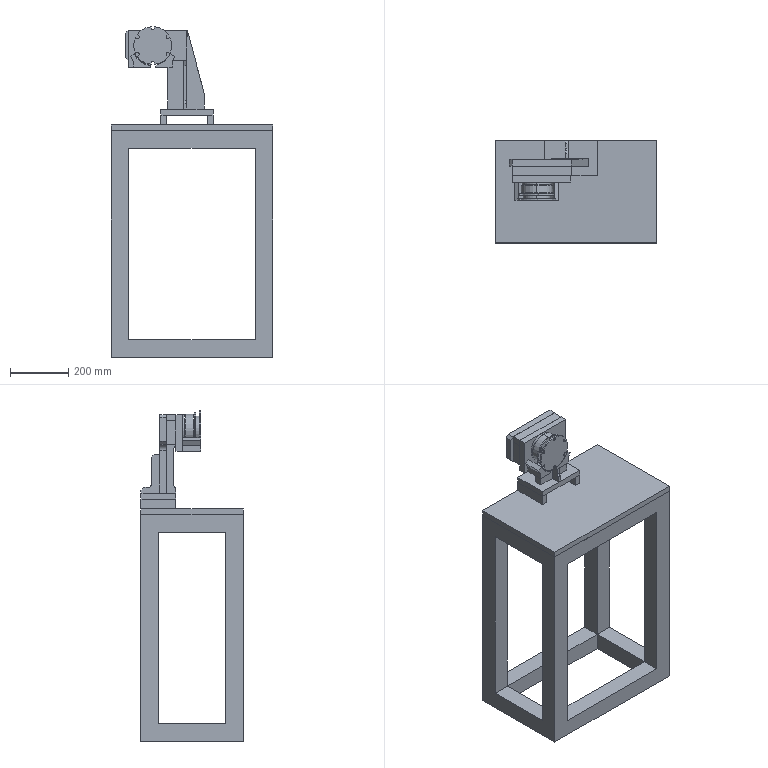Part | STEP file | Wire-arranging machine schematic | 1 solid | 191 faces | box 555 x 350.2 x 1135 mm | volume 27799243 mm3 | plane 143 | cylinder 47 | cone 1 | commonest cylinder face diameters 18 x11 10.6 x9 121.2 x6 130 x6 52 x2 68 x2